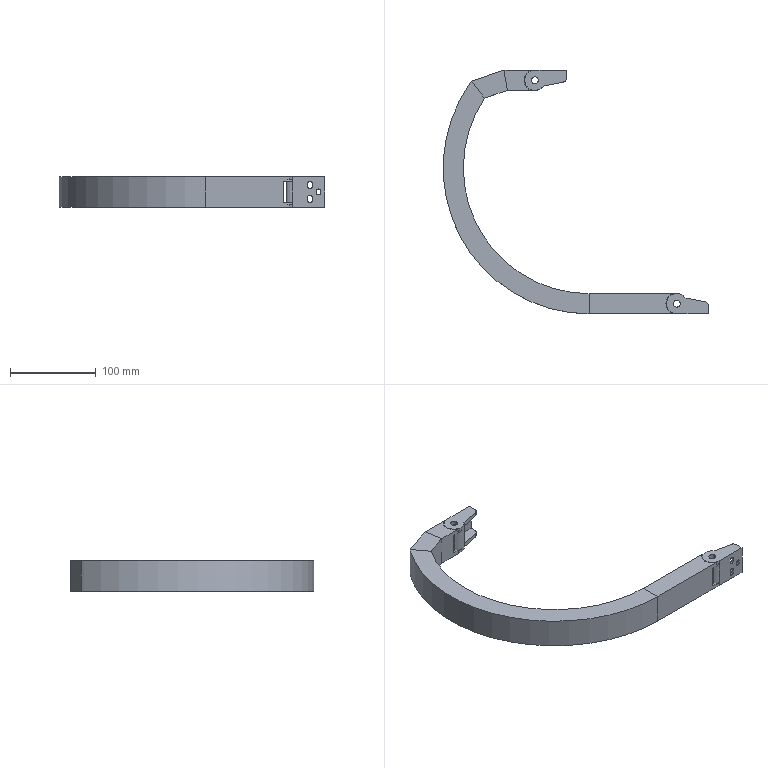Part | SolidWorks | features ICE 8, MirrorPattern 1, Sweep 1 | 3 solids | 126 faces | box 308.75 x 283.5 x 35 mm | volume 208341 mm3 | plane 76 | cylinder 48 | spline 2 | commonest cylinder face diameters 5 x18 8 x12 25 x6 10 x4 23.5 x4 292.5 x2